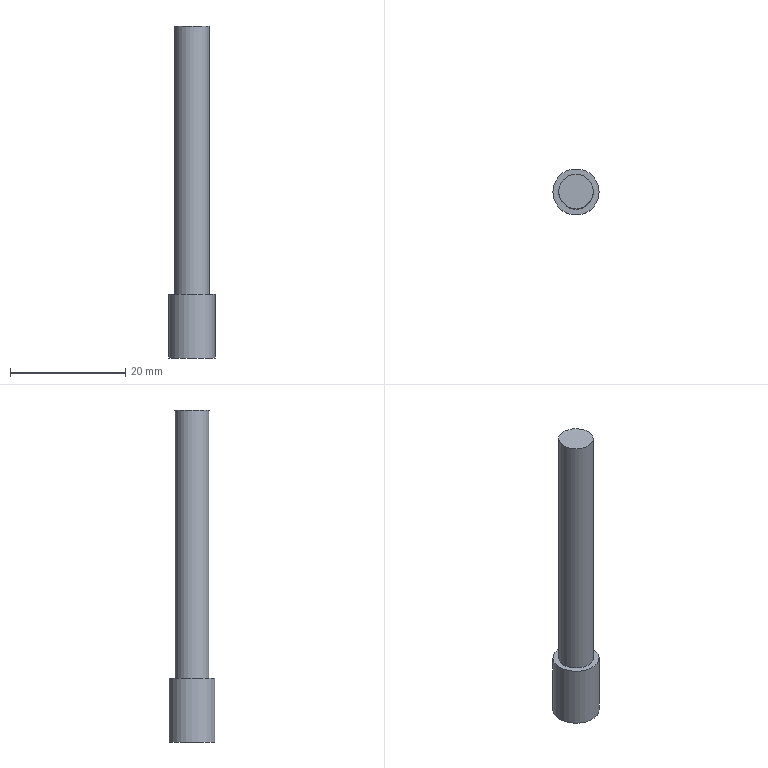Part | NX | features solid 2 | 1 solid | 5 faces | box 8 x 8 x 57.5 mm | volume 1868 mm3 | plane 3 | cylinder 2 | commonest cylinder face diameters 6 x1 8 x1
STEP:
#1=CARTESIAN_POINT('',(93.,29.5,7.5));
#2=VERTEX_POINT('',#1);
#3=CARTESIAN_POINT('',(90.,29.5,7.5));
#4=DIRECTION('',(0.,0.,1.));
#5=DIRECTION('',(1.,0.,0.));
#6=AXIS2_PLACEMENT_3D('',#3,#4,#5);
#7=CIRCLE('',#6,3.);
#8=EDGE_CURVE('',#2,#2,#7,.T.);
#9=ORIENTED_EDGE('',*,*,#8,.F.);
#10=EDGE_LOOP('',(#9));
#11=FACE_BOUND('',#10,.T.);
#12=CARTESIAN_POINT('',(87.,29.5,-39.));
#13=VERTEX_POINT('',#12);
#14=CARTESIAN_POINT('',(90.,29.5,-39.));
#15=DIRECTION('',(0.,0.,-1.));
#16=DIRECTION('',(-1.,0.,0.));
#17=AXIS2_PLACEMENT_3D('',#14,#15,#16);
#18=CIRCLE('',#17,3.);
#19=EDGE_CURVE('',#13,#13,#18,.F.);
#20=ORIENTED_EDGE('',*,*,#19,.T.);
#21=EDGE_LOOP('',(#20));
#22=FACE_BOUND('',#21,.T.);
#23=CARTESIAN_POINT('',(90.,29.5,-35.));
#24=DIRECTION('',(0.,0.,1.));
#25=DIRECTION('',(1.,0.,0.));
#26=AXIS2_PLACEMENT_3D('',#23,#24,#25);
#27=CYLINDRICAL_SURFACE('',#26,3.);
#28=ADVANCED_FACE('',(#11,#22),#27,.T.);
#29=ORIENTED_EDGE('',*,*,#8,.T.);
#30=EDGE_LOOP('',(#29));
#31=FACE_BOUND('',#30,.T.);
#32=CARTESIAN_POINT('',(90.,29.5,7.5));
#33=DIRECTION('',(0.,0.,1.));
#34=DIRECTION('',(1.,0.,0.));
#35=AXIS2_PLACEMENT_3D('',#32,#33,#34);
#36=PLANE('',#35);
#37=ADVANCED_FACE('',(#31),#36,.T.);
#38=CARTESIAN_POINT('',(86.,29.5,-39.));
#39=VERTEX_POINT('',#38);
#40=CARTESIAN_POINT('',(90.,29.5,-39.));
#41=DIRECTION('',(0.,0.,-1.));
#42=DIRECTION('',(-1.,0.,0.));
#43=AXIS2_PLACEMENT_3D('',#40,#41,#42);
#44=CIRCLE('',#43,4.);
#45=EDGE_CURVE('',#39,#39,#44,.T.);
#46=ORIENTED_EDGE('',*,*,#45,.T.);
#47=EDGE_LOOP('',(#46));
#48=FACE_BOUND('',#47,.T.);
#49=CARTESIAN_POINT('',(86.,29.5,-50.));
#50=VERTEX_POINT('',#49);
#51=CARTESIAN_POINT('',(90.,29.5,-50.));
#52=DIRECTION('',(0.,0.,-1.));
#53=DIRECTION('',(-1.,0.,0.));
#54=AXIS2_PLACEMENT_3D('',#51,#52,#53);
#55=CIRCLE('',#54,4.);
#56=EDGE_CURVE('',#50,#50,#55,.T.);
#57=ORIENTED_EDGE('',*,*,#56,.F.);
#58=EDGE_LOOP('',(#57));
#59=FACE_BOUND('',#58,.T.);
#60=CARTESIAN_POINT('',(90.,29.5,-38.));
#61=DIRECTION('',(0.,0.,-1.));
#62=DIRECTION('',(-1.,0.,0.));
#63=AXIS2_PLACEMENT_3D('',#60,#61,#62);
#64=CYLINDRICAL_SURFACE('',#63,4.);
#65=ADVANCED_FACE('',(#48,#59),#64,.T.);
#66=ORIENTED_EDGE('',*,*,#19,.F.);
#67=EDGE_LOOP('',(#66));
#68=FACE_BOUND('',#67,.T.);
#69=ORIENTED_EDGE('',*,*,#45,.F.);
#70=EDGE_LOOP('',(#69));
#71=FACE_BOUND('',#70,.T.);
#72=CARTESIAN_POINT('',(90.,29.5,-39.));
#73=DIRECTION('',(0.,0.,-1.));
#74=DIRECTION('',(-1.,0.,0.));
#75=AXIS2_PLACEMENT_3D('',#72,#73,#74);
#76=PLANE('',#75);
#77=ADVANCED_FACE('',(#68,#71),#76,.F.);
#78=ORIENTED_EDGE('',*,*,#56,.T.);
#79=EDGE_LOOP('',(#78));
#80=FACE_BOUND('',#79,.T.);
#81=CARTESIAN_POINT('',(8.802,-89.336,-50.));
#82=DIRECTION('',(0.,0.,1.));
#83=DIRECTION('',(-1.,0.,0.));
#84=AXIS2_PLACEMENT_3D('',#81,#82,#83);
#85=PLANE('',#84);
#86=ADVANCED_FACE('',(#80),#85,.F.);
#87=CLOSED_SHELL('',(#28,#37,#65,#77,#86));
#88=MANIFOLD_SOLID_BREP('',#87);
#89=(LENGTH_UNIT()NAMED_UNIT(*)SI_UNIT(.MILLI.,.METRE.));
#90=UNCERTAINTY_MEASURE_WITH_UNIT(LENGTH_MEASURE(0.00001),#89,'','');
#91=(NAMED_UNIT(*)PLANE_ANGLE_UNIT()SI_UNIT($,.RADIAN.));
#92=(NAMED_UNIT(*)SI_UNIT($,.STERADIAN.)SOLID_ANGLE_UNIT());
#93=(GEOMETRIC_REPRESENTATION_CONTEXT(3)GLOBAL_UNCERTAINTY_ASSIGNED_CONTEXT((#90))GLOBAL_UNIT_ASSIGNED_CONTEXT((#89,#91,#92))REPRESENTATION_CONTEXT('',''));
#94=ADVANCED_BREP_SHAPE_REPRESENTATION('',(#88),#93);